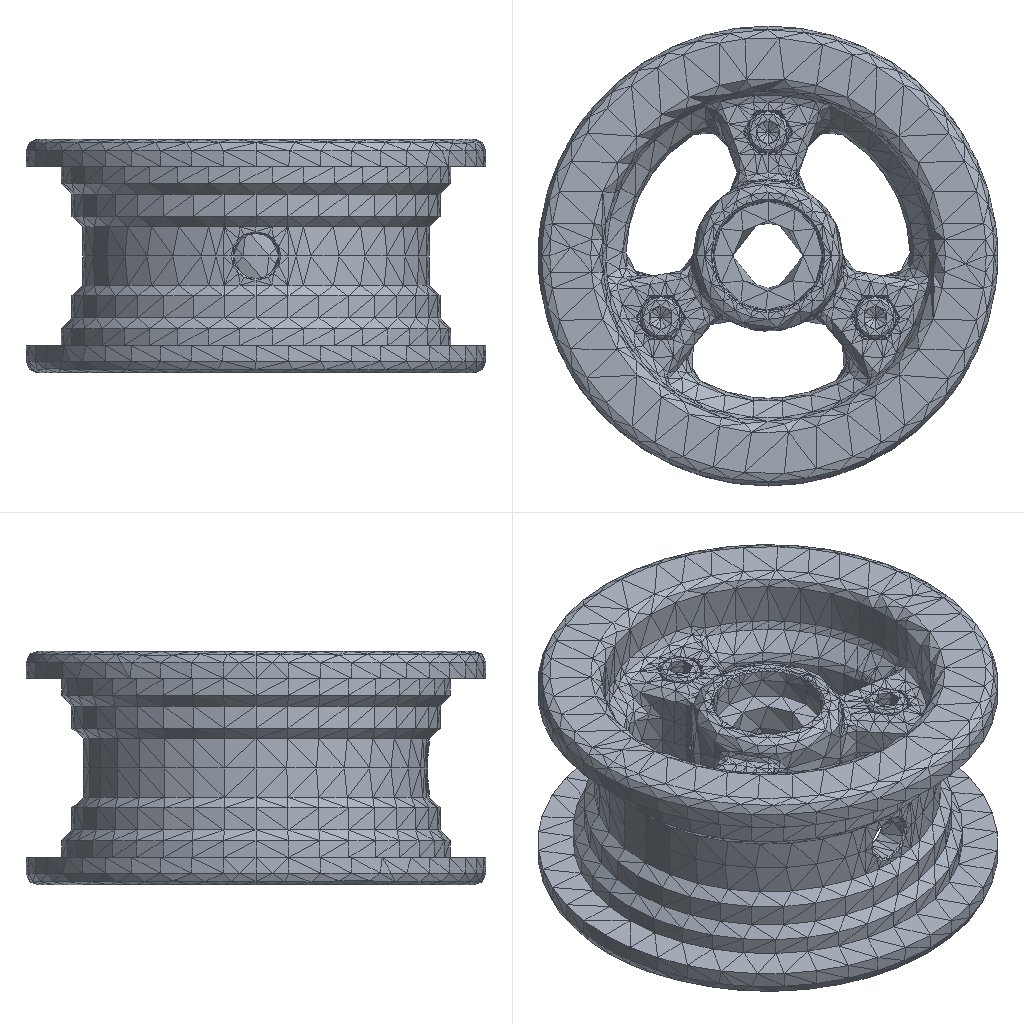Simulation study | ansys workbench
Ansys APDL input file, long lists of numbers shortened:
/batch
/config,noeldb,1     ! force off writing results to database
*get,_wallstrt,active,,time,wall
! ANSYS input file written by Workbench version 2022 R1
! File used for geometry attach:
/title,wbnew--____ (C5)
! ****** Begin Custom Load Command Snippet ******
/COM, ACT Extensions:
/COM,     LSDYNA, 2021.1
/COM,
! ****** End   Custom Load Command Snippet ******
*DIM,_wb_ProjectScratch_dir,string,248
_wb_ProjectScratch_dir(1) = ''
*DIM,_wb_SolverFiles_dir,string,248
_wb_SolverFiles_dir(1) = ''
*DIM,_wb_userfiles_dir,string,248
_wb_userfiles_dir(1) = ''
/com,--- Data in consistent NMM units. See Solving Units in the help system for more information.
/units,MPA
/nopr
/wb,file,start              !  signify a WB generated input file
/prep7
! Turn off shape checking because checks already performed inside WB mesher.
! See help system for more information.
SHPP,OFF,,NOWARN
/nolist
etcon,set             ! allow ANSYS to choose best KEYOP's for 180x elements, resets any applicable keyopt to MAPDL defaults
/com,*********** Nodes for the whole assembly ***********
nblock,3,,38121
(1i9,3e20.9e3)
        1    -7.914531287E+01    -4.780604649E+00     3.826096569E+01
! (34655 more lines like these left out)
-1
/com,*********** Nodes for all Remote Points ***********
nblock,3
(1i9,3e20.9e3)
    34657    -5.164828464E+01     3.178927256E+01     2.986739921E+01
-1
/wb,elem,start            !  set before creation of elements
/com,*********** Elements for Body 1 "Wheel Hub|Pah4" ***********
et,1,187
eblock,19,solid,,6596
(19i9)
        1        1        1        1        0        0        0        0       10        0     5341    10933    11707    12259    11913    16847    20987    16852    16849
! (13191 more lines like these left out)
-1
/com,*********** Elements for Body 2 "Wheel Hub|Pah4[2]" ***********
et,2,187
eblock,19,solid,,6596
(19i9)
        2        2        2        2        0        0        0        0       10        0    11937    23119    23893    24445    24099    29033    33173    29038    29035
! (13191 more lines like these left out)
-1
/com,*********** Elements for Body 3 "socket head cap screw_am32323_PreviewCfg|____1" ***********
et,3,187
eblock,19,solid,,671
(19i9)
        3        3        3        3        0        0        0        0       10        0     2890     5582     5699     5789     5773     5900     6546     5906     5904
! (1341 more lines like these left out)
-1
/com,*********** Elements for Body 4 "socket head cap screw_am32323_PreviewCfg|____1[2]" ***********
et,4,187
eblock,19,solid,,671
(19i9)
        4        4        4        4        0        0        0        0       10        0        1       12      129      219      203      330      976      336      334
! (1341 more lines like these left out)
-1
/com,*********** Elements for Body 5 "socket head cap screw_am32323_PreviewCfg|____1[3]" ***********
et,5,187
eblock,19,solid,,671
(19i9)
        5        5        5        5        0        0        0        0       10        0     3561     6868     6985     7075     7059     7186     7832     7192     7190
! (1341 more lines like these left out)
-1
/com,*********** Elements for Body 6 "hex nut style 1_am333_PreviewCfg|____1" ***********
et,6,187
eblock,19,solid,,1109
(19i9)
        6        6        6        6        0        0        0        0       10        0      672     1594     1655     1617     1649     3300     3384     3296     3298
! (2217 more lines like these left out)
-1
/com,*********** Elements for Body 7 "hex nut style 1_am333_PreviewCfg|____1[2]" ***********
et,7,187
eblock,19,solid,,1109
(19i9)
        7        7        7        7        0        0        0        0       10        0     1781     3736     3797     3759     3791     5442     5526     5438     5440
! (2217 more lines like these left out)
-1
/com,*********** Elements for Body 8 "hex nut style 1_am333_PreviewCfg|____1[3]" ***********
et,8,187
eblock,19,solid,,1109
(19i9)
        8        8        8        8        0        0        0        0       10        0     4232     8450     8511     8473     8505    10156    10240    10152    10154
! (2217 more lines like these left out)
-1
/wb,elem,end               !  done creating elements
/com,*********** Send User Defined Coordinate System(s) ***********
csys,0
toffst,273.15,  ! Temperature offset from absolute zero
/com,*********** Set Reference Temperature ***********
tref,22.
/wb,mat,start              !  starting to send materials
/com,*********** Send Materials ***********
Temperature = 'TEMP' ! Temperature
MP,DENS,1,7.85e-09,	! tonne mm^-3
MP,ALPX,1,1.2e-05,	! C^-1
MP,C,1,434000000,	! mm^2 s^-2 C^-1
MP,KXX,1,60.5,	! tonne mm s^-3 C^-1
MP,RSVX,1,0.00017,	! ohm mm
MP,EX,1,200000,	! tonne s^-2 mm^-1
MP,NUXY,1,0.3,
MP,MURX,1,10000,
Temperature = 'TEMP' ! Temperature
MP,DENS,2,7.85e-09,	! tonne mm^-3
MP,ALPX,2,1.2e-05,	! C^-1
MP,C,2,434000000,	! mm^2 s^-2 C^-1
MP,KXX,2,60.5,	! tonne mm s^-3 C^-1
MP,RSVX,2,0.00017,	! ohm mm
MP,EX,2,200000,	! tonne s^-2 mm^-1
MP,NUXY,2,0.3,
MP,MURX,2,10000,
Temperature = 'TEMP' ! Temperature
MP,DENS,3,7.85e-09,	! tonne mm^-3
MP,ALPX,3,1.2e-05,	! C^-1
MP,C,3,434000000,	! mm^2 s^-2 C^-1
MP,KXX,3,60.5,	! tonne mm s^-3 C^-1
MP,RSVX,3,0.00017,	! ohm mm
MP,EX,3,200000,	! tonne s^-2 mm^-1
MP,NUXY,3,0.3,
MP,MURX,3,10000,
Temperature = 'TEMP' ! Temperature
MP,DENS,4,7.85e-09,	! tonne mm^-3
MP,ALPX,4,1.2e-05,	! C^-1
MP,C,4,434000000,	! mm^2 s^-2 C^-1
MP,KXX,4,60.5,	! tonne mm s^-3 C^-1
MP,RSVX,4,0.00017,	! ohm mm
MP,EX,4,200000,	! tonne s^-2 mm^-1
MP,NUXY,4,0.3,
MP,MURX,4,10000,
Temperature = 'TEMP' ! Temperature
MP,DENS,5,7.85e-09,	! tonne mm^-3
MP,ALPX,5,1.2e-05,	! C^-1
MP,C,5,434000000,	! mm^2 s^-2 C^-1
MP,KXX,5,60.5,	! tonne mm s^-3 C^-1
MP,RSVX,5,0.00017,	! ohm mm
MP,EX,5,200000,	! tonne s^-2 mm^-1
MP,NUXY,5,0.3,
MP,MURX,5,10000,
Temperature = 'TEMP' ! Temperature
MP,DENS,6,7.85e-09,	! tonne mm^-3
MP,ALPX,6,1.2e-05,	! C^-1
MP,C,6,434000000,	! mm^2 s^-2 C^-1
MP,KXX,6,60.5,	! tonne mm s^-3 C^-1
MP,RSVX,6,0.00017,	! ohm mm
MP,EX,6,200000,	! tonne s^-2 mm^-1
MP,NUXY,6,0.3,
MP,MURX,6,10000,
Temperature = 'TEMP' ! Temperature
MP,DENS,7,7.85e-09,	! tonne mm^-3
MP,ALPX,7,1.2e-05,	! C^-1
MP,C,7,434000000,	! mm^2 s^-2 C^-1
MP,KXX,7,60.5,	! tonne mm s^-3 C^-1
MP,RSVX,7,0.00017,	! ohm mm
MP,EX,7,200000,	! tonne s^-2 mm^-1
MP,NUXY,7,0.3,
MP,MURX,7,10000,
Temperature = 'TEMP' ! Temperature
MP,DENS,8,7.85e-09,	! tonne mm^-3
MP,ALPX,8,1.2e-05,	! C^-1
MP,C,8,434000000,	! mm^2 s^-2 C^-1
MP,KXX,8,60.5,	! tonne mm s^-3 C^-1
MP,RSVX,8,0.00017,	! ohm mm
MP,EX,8,200000,	! tonne s^-2 mm^-1
MP,NUXY,8,0.3,
MP,MURX,8,10000,
/wb,mat,end                !  done sending materials
!************************* Model Summary ********************
!Wheel Hub|Pah4,	结构钢,	matid,	1
!Wheel Hub|Pah4[2],	结构钢,	matid,	2
!socket head cap screw_am32323_PreviewCfg|____1,	结构钢,	matid,	3
!socket head cap screw_am32323_PreviewCfg|____1[2],	结构钢,	matid,	4
!socket head cap screw_am32323_PreviewCfg|____1[3],	结构钢,	matid,	5
!hex nut style 1_am333_PreviewCfg|____1,	结构钢,	matid,	6
!hex nut style 1_am333_PreviewCfg|____1[2],	结构钢,	matid,	7
!hex nut style 1_am333_PreviewCfg|____1[3],	结构钢,	matid,	8
!************************* End Model Summary ********************
! get the diagonal of the bounding box. Needed later for other things
*get,_xmin,node,,mnloc,x
*get,_ymin,node,,mnloc,y
*get,_zmin,node,,mnloc,z
*get,_xmax,node,,mxloc,x
*get,_ymax,node,,mxloc,y
*get,_zmax,node,,mxloc,z
_ASMDIAG=(_xmax-_xmin)*(_xmax-_xmin)+(_ymax-_ymin)*(_ymax-_ymin)+(_zmax-_zmin)*(_zmax-_zmin)
_ASMDIAG=SQRT(_ASMDIAG)
/wb,contact,start          !  starting to send contact
/com,*********** Create Contact "接触区域" ***********
/com,            Real Constant Set For Above Contact Is 10 & 9
*set,tid,10
*set,cid,9
r,tid
r,cid
et,tid,170
et,cid,174
eblock,10,,,292
(15i9)
    27844       10       10       10        0    10309    10311    10313    10313    12419    12436    10313    12420
! (291 more lines like these left out)
-1
eblock,10,,,292
(15i9)
    28136        9        9        9        0    10309    10311    10313    10313    12419    12436    10313    12420
! (291 more lines like these left out)
-1
eblock,10,,,292
(15i9)
    28428        9       10        9        0    22510    22980    23548    23548    24717    28080    23548    24718
! (291 more lines like these left out)
-1
eblock,10,,,292
(15i9)
    28720       10        9       10        0    22510    22980    23548    23548    24717    28080    23548    24718
! (291 more lines like these left out)
-1
keyo,cid,8,2               ! auto create asymmetric contact (from Program Controlled setting)
keyo,cid,10,0              ! adjust contact stiffness each NR iteration (from Program Controlled setting)
keyo,cid,12,5              ! bonded always
keyo,cid,18,1              ! small sliding turned on by application
keyo,cid,2,0               ! augmented Lagrange (from Program Controlled setting)
keyo,cid,4,0               ! on Gauss point (from Program Controlled setting)
keyo,cid,9,1               ! ignore initial gaps/penetration
keyo,cid,7,0               ! No Prediction
rmod,tid,3,10.      ! FKN
rmod,tid,5,0.       ! ICONT
rmod,tid,6,0.       ! PINB
rmod,tid,10,0.      ! CNOF
rmod,tid,12,0.      ! FKT
rmod,tid,36,47      ! WB DSID
rmod,cid,3,10.      ! FKN
rmod,cid,5,0.       ! ICONT
rmod,cid,6,0.       ! PINB
rmod,cid,10,0.      ! CNOF
rmod,cid,12,0.      ! FKT
rmod,cid,36,47      ! WB DSID
/com,*********** Create Contact "接触区域 2" ***********
/com,            Real Constant Set For Above Contact Is 12 & 11
*set,tid,12
*set,cid,11
r,tid
r,cid
et,tid,170
et,cid,174
eblock,10,,,78
(15i9)
    29012       12       12       12        0    10732    10733    11268    11268    15538    15545    11268    15539
! (77 more lines like these left out)
-1
eblock,10,,,78
(15i9)
    29090       11       11       11        0    10732    10733    11268    11268    15538    15545    11268    15539
! (77 more lines like these left out)
-1
eblock,10,,,120
(15i9)
    29168       11       12       11        0     5684     5683     5587     5587     6468     5941     5587     5942
! (119 more lines like these left out)
-1
eblock,10,,,120
(15i9)
    29288       12       11       12        0     5684     5683     5587     5587     6468     5941     5587     5942
! (119 more lines like these left out)
-1
keyo,cid,8,2               ! auto create asymmetric contact (from Program Controlled setting)
keyo,cid,10,0              ! adjust contact stiffness each NR iteration (from Program Controlled setting)
keyo,cid,12,5              ! bonded always
keyo,cid,18,1              ! small sliding turned on by application
keyo,cid,2,0               ! augmented Lagrange (from Program Controlled setting)
keyo,cid,4,0               ! on Gauss point (from Program Controlled setting)
keyo,cid,9,1               ! ignore initial gaps/penetration
keyo,cid,7,0               ! No Prediction
rmod,tid,3,10.      ! FKN
rmod,tid,5,0.       ! ICONT
rmod,tid,6,0.       ! PINB
rmod,tid,10,0.      ! CNOF
rmod,tid,12,0.      ! FKT
rmod,tid,36,50      ! WB DSID
rmod,cid,3,10.      ! FKN
rmod,cid,5,0.       ! ICONT
rmod,cid,6,0.       ! PINB
rmod,cid,10,0.      ! CNOF
rmod,cid,12,0.      ! FKT
rmod,cid,36,50      ! WB DSID
/com,*********** Create Contact "接触区域 3" ***********
/com,            Real Constant Set For Above Contact Is 14 & 13
*set,tid,14
*set,cid,13
r,tid
r,cid
et,tid,170
et,cid,174
eblock,10,,,78
(15i9)
    29408       14       14       14        0    10740    11282    11277    11277    15595    19068    11277    15594
! (77 more lines like these left out)
-1
eblock,10,,,78
(15i9)
    29486       13       13       13        0    10740    11282    11277    11277    15595    19068    11277    15594
! (77 more lines like these left out)
-1
eblock,10,,,120
(15i9)
    29564       13       14       13        0      114      113       17       17      898      371       17      372
! (119 more lines like these left out)
-1
eblock,10,,,120
(15i9)
    29684       14       13       14        0      114      113       17       17      898      371       17      372
! (119 more lines like these left out)
-1
keyo,cid,8,2               ! auto create asymmetric contact (from Program Controlled setting)
keyo,cid,10,0              ! adjust contact stiffness each NR iteration (from Program Controlled setting)
keyo,cid,12,5              ! bonded always
keyo,cid,18,1              ! small sliding turned on by application
keyo,cid,2,0               ! augmented Lagrange (from Program Controlled setting)
keyo,cid,4,0               ! on Gauss point (from Program Controlled setting)
keyo,cid,9,1               ! ignore initial gaps/penetration
keyo,cid,7,0               ! No Prediction
rmod,tid,3,10.      ! FKN
rmod,tid,5,0.       ! ICONT
rmod,tid,6,0.       ! PINB
rmod,tid,10,0.      ! CNOF
rmod,tid,12,0.      ! FKT
rmod,tid,36,53      ! WB DSID
rmod,cid,3,10.      ! FKN
rmod,cid,5,0.       ! ICONT
rmod,cid,6,0.       ! PINB
rmod,cid,10,0.      ! CNOF
rmod,cid,12,0.      ! FKT
rmod,cid,36,53      ! WB DSID
/com,*********** Create Contact "接触区域 4" ***********
/com,            Real Constant Set For Above Contact Is 16 & 15
*set,tid,16
*set,cid,15
r,tid
r,cid
et,tid,170
et,cid,174
eblock,10,,,96
(15i9)
    29804       16       16       16        0    10722    11519    10954    10954    15475    17014    10954    15472
! (95 more lines like these left out)
-1
eblock,10,,,96
(15i9)
    29900       15       15       15        0    10722    11519    10954    10954    15475    17014    10954    15472
! (95 more lines like these left out)
-1
eblock,10,,,120
(15i9)
    29996       15       16       15        0     6970     6969     6873     6873     7754     7227     6873     7228
! (119 more lines like these left out)
-1
eblock,10,,,120
(15i9)
    30116       16       15       16        0     6970     6969     6873     6873     7754     7227     6873     7228
! (119 more lines like these left out)
-1
keyo,cid,8,2               ! auto create asymmetric contact (from Program Controlled setting)
keyo,cid,10,0              ! adjust contact stiffness each NR iteration (from Program Controlled setting)
keyo,cid,12,5              ! bonded always
keyo,cid,18,1              ! small sliding turned on by application
keyo,cid,2,0               ! augmented Lagrange (from Program Controlled setting)
keyo,cid,4,0               ! on Gauss point (from Program Controlled setting)
keyo,cid,9,1               ! ignore initial gaps/penetration
keyo,cid,7,0               ! No Prediction
rmod,tid,3,10.      ! FKN
rmod,tid,5,0.       ! ICONT
rmod,tid,6,0.       ! PINB
rmod,tid,10,0.      ! CNOF
rmod,tid,12,0.      ! FKT
rmod,tid,36,56      ! WB DSID
rmod,cid,3,10.      ! FKN
rmod,cid,5,0.       ! ICONT
rmod,cid,6,0.       ! PINB
rmod,cid,10,0.      ! CNOF
rmod,cid,12,0.      ! FKT
rmod,cid,36,56      ! WB DSID
/com,*********** Create Contact "接触区域 5" ***********
/com,            Real Constant Set For Above Contact Is 18 & 17
*set,tid,18
*set,cid,17
r,tid
r,cid
et,tid,170
et,cid,174
eblock,10,,,12
(15i9)
    30236       18       18       18        0    22918    22919    23454    23454    27724    27731    23454    27725
! (11 more lines like these left out)
-1
eblock,10,,,12
(15i9)
    30248       17       17       17        0    22918    22919    23454    23454    27724    27731    23454    27725
! (11 more lines like these left out)
-1
eblock,10,,,154
(15i9)
    30260       17       18       17        0     1451     1509     1559     1559     2687     2875     1559     2689
! (153 more lines like these left out)
-1
eblock,10,,,154
(15i9)
    30414       18       17       18        0     1451     1509     1559     1559     2687     2875     1559     2689
! (153 more lines like these left out)
-1
keyo,cid,8,2               ! auto create asymmetric contact (from Program Controlled setting)
keyo,cid,10,0              ! adjust contact stiffness each NR iteration (from Program Controlled setting)
keyo,cid,12,5              ! bonded always
keyo,cid,18,1              ! small sliding turned on by application
keyo,cid,2,0               ! augmented Lagrange (from Program Controlled setting)
keyo,cid,4,0               ! on Gauss point (from Program Controlled setting)
keyo,cid,9,1               ! ignore initial gaps/penetration
keyo,cid,7,0               ! No Prediction
rmod,tid,3,10.      ! FKN
rmod,tid,5,0.       ! ICONT
rmod,tid,6,0.       ! PINB
rmod,tid,10,0.      ! CNOF
rmod,tid,12,0.      ! FKT
rmod,tid,36,59      ! WB DSID
rmod,cid,3,10.      ! FKN
rmod,cid,5,0.       ! ICONT
rmod,cid,6,0.       ! PINB
rmod,cid,10,0.      ! CNOF
rmod,cid,12,0.      ! FKT
rmod,cid,36,59      ! WB DSID
/com,*********** Create Contact "接触区域 6" ***********
/com,            Real Constant Set For Above Contact Is 20 & 19
*set,tid,20
*set,cid,19
r,tid
r,cid
et,tid,170
et,cid,174
eblock,10,,,19
(15i9)
    30568       20       20       20        0    22908    23705    23140    23140    27661    29200    23140    27658
! (18 more lines like these left out)
-1
eblock,10,,,19
(15i9)
    30587       19       19       19        0    22908    23705    23140    23140    27661    29200    23140    27658
! (18 more lines like these left out)
-1
eblock,10,,,147
(15i9)
    30606       19       20       19        0     3593     3651     3701     3701     4829     5017     3701     4831
! (146 more lines like these left out)
-1
eblock,10,,,147
(15i9)
    30753       20       19       20        0     3593     3651     3701     3701     4829     5017     3701     4831
! (146 more lines like these left out)
-1
keyo,cid,8,2               ! auto create asymmetric contact (from Program Controlled setting)
keyo,cid,10,0              ! adjust contact stiffness each NR iteration (from Program Controlled setting)
keyo,cid,12,5              ! bonded always
keyo,cid,18,1              ! small sliding turned on by application
keyo,cid,2,0               ! augmented Lagrange (from Program Controlled setting)
keyo,cid,4,0               ! on Gauss point (from Program Controlled setting)
keyo,cid,9,1               ! ignore initial gaps/penetration
keyo,cid,7,0               ! No Prediction
rmod,tid,3,10.      ! FKN
rmod,tid,5,0.       ! ICONT
rmod,tid,6,0.       ! PINB
rmod,tid,10,0.      ! CNOF
rmod,tid,12,0.      ! FKT
rmod,tid,36,62      ! WB DSID
rmod,cid,3,10.      ! FKN
rmod,cid,5,0.       ! ICONT
rmod,cid,6,0.       ! PINB
rmod,cid,10,0.      ! CNOF
rmod,cid,12,0.      ! FKT
rmod,cid,36,62      ! WB DSID
/com,*********** Create Contact "接触区域 7" ***********
/com,            Real Constant Set For Above Contact Is 22 & 21
*set,tid,22
*set,cid,21
r,tid
r,cid
et,tid,170
et,cid,174
eblock,10,,,12
(15i9)
    30900       22       22       22        0    22926    23468    23463    23463    27781    31254    23463    27780
! (11 more lines like these left out)
-1
eblock,10,,,12
(15i9)
    30912       21       21       21        0    22926    23468    23463    23463    27781    31254    23463    27780
! (11 more lines like these left out)
-1
eblock,10,,,154
(15i9)
    30924       21       22       21        0     8307     8365     8415     8415     9543     9731     8415     9545
! (153 more lines like these left out)
-1
eblock,10,,,154
(15i9)
    31078       22       21       22        0     8307     8365     8415     8415     9543     9731     8415     9545
! (153 more lines like these left out)
-1
keyo,cid,8,2               ! auto create asymmetric contact (from Program Controlled setting)
keyo,cid,10,0              ! adjust contact stiffness each NR iteration (from Program Controlled setting)
keyo,cid,12,5              ! bonded always
keyo,cid,18,1              ! small sliding turned on by application
keyo,cid,2,0               ! augmented Lagrange (from Program Controlled setting)
keyo,cid,4,0               ! on Gauss point (from Program Controlled setting)
keyo,cid,9,1               ! ignore initial gaps/penetration
keyo,cid,7,0               ! No Prediction
rmod,tid,3,10.      ! FKN
rmod,tid,5,0.       ! ICONT
rmod,tid,6,0.       ! PINB
rmod,tid,10,0.      ! CNOF
rmod,tid,12,0.      ! FKT
rmod,tid,36,65      ! WB DSID
rmod,cid,3,10.      ! FKN
rmod,cid,5,0.       ! ICONT
rmod,cid,6,0.       ! PINB
rmod,cid,10,0.      ! CNOF
rmod,cid,12,0.      ! FKT
rmod,cid,36,65      ! WB DSID
nsel,all
esel,all
/wb,contact,end            !  done creating contacts
/golist
/wb,load,start             !  starting to send loads
/com,*********** Fixed Supports ***********
CMBLOCK,_FIXEDSU,NODE,      538
(8i10)
        59        60        61        62        63        64        75        76
! (67 more lines like these left out)
cmsel,s,_FIXEDSU
d,all,all
nsel,all
/com,*********** Create Remote Point "内部远程点" ***********
! -------- Remote Point Used by "力矩" --------
*set,tid,24
*set,cid,23
et,cid,174
et,tid,170
keyo,tid,2,1               ! Don't fix the pilot node
keyo,tid,4,111111
keyo,cid,12,5              ! Bonded Contact
keyo,cid,4,1               ! Deformable RBE3 style load
keyo,cid,2,2               ! MPC style contact
eblock,10,,,322
(15i9)
    31232       23       23       23        0    10743    10662    10759    10759    14971    14972    10759    15611
! (321 more lines like these left out)
-1
*set,_npilot,34657
_npilot76=_npilot
type,tid
mat ,cid
real,cid
tshape,pilo
en,31554,_npilot
tshape
/com,*********** Construct Moment Using Remote Attachment ***********
/gst,on,on
fini
*get,_numnode,node,0,count
*get,_numelem,elem,0,count
*get, _MAXELEMNUM, elem, 0, NUM, MAX
*get, _MAXNODENUM, node, 0, NUM, MAX
*get, _MAXELEMTYPE, etyp, 0, NUM, MAX
*get, _MAXREALCONST, real, 0, NUM, MAX
/go
/wb,load,end               !  done creating loads
/com,--- Number of total nodes = %_numnode%
/com,--- Number of contact elements = 3710
/com,--- Number of spring elements = 0
/com,--- Number of bearing elements = 0
/com,--- Number of solid elements = 18532
/com,--- Number of condensed parts = 0
/com,--- Number of total elements = %_numelem%
*get,_wallbsol,active,,time,wall
/com,****************************************************************************
/com,*************************    SOLUTION       ********************************
/com,****************************************************************************
/solu
antype,0                   ! static analysis
_thickRatio=  1     ! Ratio of thick parts in the model
eqsl,pcg,1e-8,,,,,,1
cntr,print,1               ! print out contact info and also make no initial contact an error
dmpoption,emat,no             ! Don't combine emat file for DANSYS
dmpoption,esav,no             ! Don't combine esav file for DANSYS
nldiag,cont,iter           ! print out contact info each equilibrium iteration
rescontrol,,none                 ! Do not keep any restart files
/com,****************************************************
/com,******************* SOLVE FOR LS 1 OF 1 ****************
nsel,s,node,,34657
f,all,mx,0.
f,all,my,0.
f,all,mz,5000.
nsel,all
/nopr
/gopr
nsub,1,1,1
time,1.
outres,erase
outres,all,none
outres,nsol,all,
outres,rsol,all
outres,eangl,all
outres,etmp,all
outres,veng,all
outres,strs,all,
outres,epel,all,
outres,eppl,all,
outres,cont,all,
! *********** WB SOLVE COMMAND ***********
! check interactive state
*get,ANSINTER_,active,,int
*if,ANSINTER_,ne,0,then
/eof
*endif
solve
/com *************** Write FE CONNECTORS *********
CEWRITE,file,ce,,INTE
/com,****************************************************
/com,*************** FINISHED SOLVE FOR LS 1 *************
*get,_wallasol,active,,time,wall
/nopr
*get,_numnode,node,0,count
*get,_numelem,elem,0,count
*get, _MAXELEMNUM, elem, 0, NUM, MAX
*get, _MAXNODENUM, node, 0, NUM, MAX,,,INTERNAL
*get, _MAXELEMTYPE, etyp, 0, NUM, MAX
*get, _MAXREALCONST, real, 0, NUM, MAX
/gopr
*get,_PCGITER,active,,solu,cgiter
/post1
xmlo,ENCODING,ISO-8859-1
xmlo,parm
/xml,parm,xml
fini
/gopr
*get,_walldone,active,,time,wall
_preptime=(_wallbsol-_wallstrt)*3600
_solvtime=(_wallasol-_wallbsol)*3600
_posttime=(_walldone-_wallasol)*3600
_totaltim=(_walldone-_wallstrt)*3600
*get,_dlbratio,active,0,solu,dlbr
*get,_combtime,active,0,solu,comb
*get,_ssmode,active,0,solu,ssmm
*get,_ndofs,active,0,solu,ndof
*get,_sol_end_time,active,0,set,time
*if,_sol_end_time,eq,1.,then
/fclean				!clean distributed files
*endif
/com,--- Total number of nodes = %_numnode%
/com,--- Total number of elements = %_numelem%
/com,--- Element load balance ratio = %_dlbratio%
/com,--- Time to combine distributed files = %_combtime%
/com,--- Sparse memory mode = %_ssmode%
/com,--- Number of DOF = %_ndofs%
/wb,file,end               ! done with WB generated input